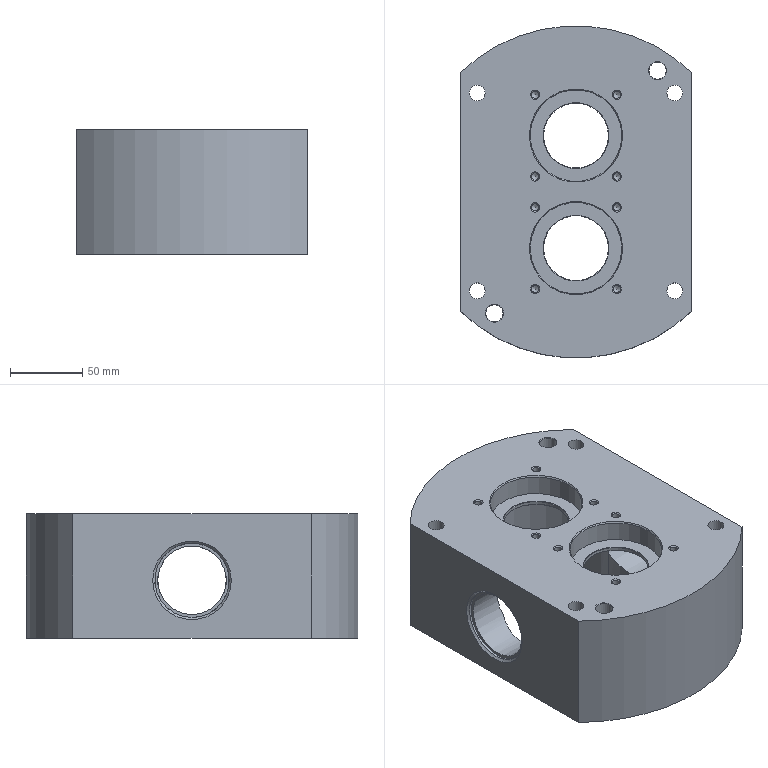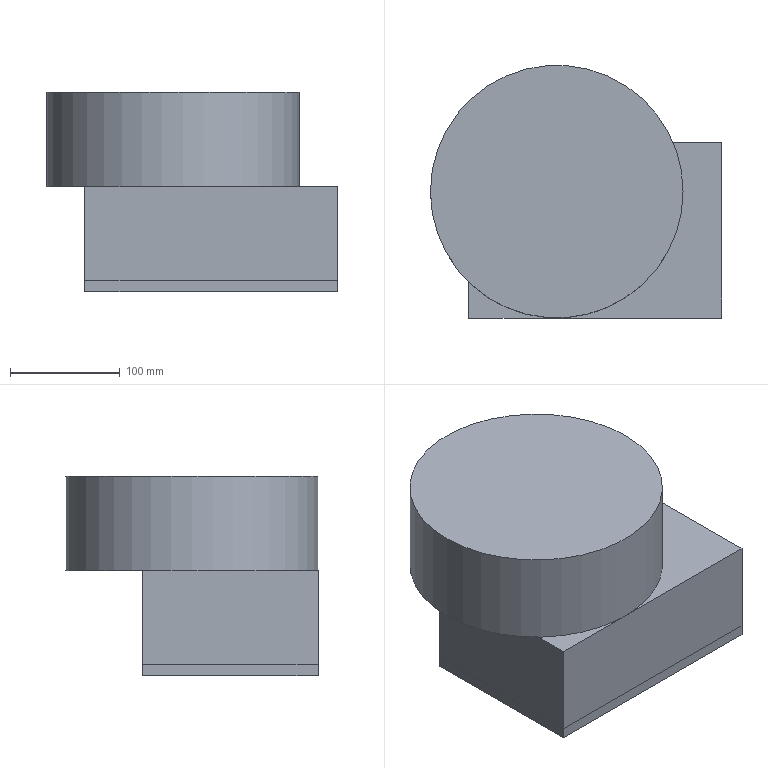CAM job | NX | 3+2 milling, drilling | part box 160 x 230 x 86 mm | stock box 265 x 230 x 182 mm
Tools:
number,name,description,diameter,corner_radius,flute_length,length,flutes
2,D50,Milling Tool-5 Parameters,50.0,0.0,50.0,75.0,2
10,D10,Milling Tool-5 Parameters,10.0,0.0,50.0,75.0,2
11,D10JING,Milling Tool-5 Parameters,10.0,0.0,50.0,75.0,2
7,D6A45,Milling Tool-5 Parameters,6.0,0.0,50.0,75.0,2
1,ZXZ,Milling Tool-5 Parameters,6.0,0.0,50.0,75.0,2
9,11.0ZT,Drilling Tool,11.0,0.0,35.0,50.0,2
8,11.8ZT,Drilling Tool,11.8,0.0,35.0,50.0,2
18,12.0JD,Milling Tool-5 Parameters,8.0,0.0,30.0,30.0,4
15,5.0ZT,Drilling Tool,5.0,0.0,35.0,50.0,2
16,6.8ZT,Drilling Tool,6.8,0.0,35.0,50.0,2
5,D25R0.5,Milling Tool-5 Parameters,25.0,0.5,50.0,75.0,2
12,D12,Milling Tool-5 Parameters,12.0,0.0,50.0,75.0,2
14,M6,Milling Tool-5 Parameters,5.0,0.0,30.0,30.0,4
18,M8,Milling Tool-5 Parameters,6.8,0.0,30.0,30.0,4
Operations:
program,operation,operation_type,tool,method,geometry_group,spindle_rpm,surface_speed,feed_per_tooth,feed_cut,feed_plunge,cut_length_mm,path_length_mm,cut_time_min,machine_time_min
1,FLOOR_WALL,VolumeBased25DMillingOperation,D50,METHOD,A,1200.0,188.0,0.8333,2000.0,1000.0,83660.764,101099.88,42.13,43.874
1,FLOOR_WALL_COPY,VolumeBased25DMillingOperation,D50,METHOD,A,2500.0,392.0,0.2,1000.0,1000.0,1038.906,1162.906,1.039,1.051
1,HOLE_MILLING,CylinderMilling,D10,METHOD,A,3000.0,94.0,0.3667,2200.0,100.0,6416.122,6548.622,2.916,2.93
1,HOLE_MILLING_COPY,CylinderMilling,D10,METHOD,A,3000.0,94.0,0.3667,2200.0,100.0,7693.753,7859.253,3.497,3.514
1,HOLE_MILLING_COPY_1,CylinderMilling,D10JING,METHOD,A,5000.0,157.0,0.1,1000.0,100.0,175.612,311.612,0.1756,0.1892
1,HOLE_MILLING_COPY_1_COPY,CylinderMilling,D10JING,METHOD,A,5000.0,157.0,0.1,1000.0,100.0,163.983,359.983,0.164,0.1836
1,PLANAR_MILL,PlanarMilling,D6A45,METHOD,A,7500.0,141.0,0.0833,1250.0,100.0,350.346,691.746,0.2803,0.3144
1,PLANAR_MILL_COPY,PlanarMilling,D6A45,METHOD,A,7500.0,141.0,0.0833,1250.0,100.0,483.313,611.313,0.3867,0.3995
2,DRILLING,Operation,ZXZ,METHOD,B,5000.0,94.0,0.025,250.0,0.0,64.0,820.526,0.256,0.3317
2,DRILLING_COPY,Operation,11.0ZT,METHOD,B,2000.0,56.0,0.0375,150.0,0.0,377.219,1234.536,2.515,2.6
2,DRILLING_COPY_COPY,Operation,11.8ZT,METHOD,B,2000.0,56.0,0.0375,150.0,0.0,188.09,641.67,1.254,1.299
2,DRILLING_COPY_COPY_COPY,Operation,12.0JD,METHOD,B,800.0,20.0,0.0125,40.0,0.0,179.0,623.49,4.475,4.519
2,DRILLING_COPY_COPY_1,Operation,5.0ZT,METHOD,B,2000.0,56.0,0.0375,150.0,0.0,140.017,687.555,0.9334,0.9882
2,DRILLING_COPY_2_COPY_COPY_1_COPY,Operation,M6,METHOD,B,200.0,3.0,0.0013,1.0,0.0,128.0,663.521,128.0,128.054
2,HOLE_MILLING_COPY_COPY,CylinderMilling,D10,METHOD,B,3000.0,94.0,0.3667,2200.0,100.0,24671.677,24898.677,11.214,11.237
2,HOLE_MILLING_COPY_COPY_COPY,CylinderMilling,D10,METHOD,B,3000.0,94.0,0.3667,2200.0,100.0,10167.626,10429.626,4.622,4.648
2,ZLEVEL_PROFILE,ZLevelMilling,D10JING,METHOD,B,5000.0,157.0,0.125,1250.0,100.0,239.51,498.755,0.1916,0.2175
2,PLANAR_MILL_COPY_COPY,PlanarMilling,D6A45,METHOD,B,7500.0,141.0,0.0833,1250.0,100.0,807.404,2282.468,0.6459,0.7934
2,PLANAR_MILL_COPY_COPY_COPY,PlanarMilling,D6A45,METHOD,B,7500.0,141.0,0.0833,1250.0,100.0,287.856,536.813,0.2303,0.2552
2,刀补,CylinderMilling,D10JING,METHOD,B,5000.0,157.0,0.1,1000.0,100.0,357.211,608.344,0.3572,0.3823
3,FLOOR_WALL_COPY_1,VolumeBased25DMillingOperation,D50,METHOD,C,1200.0,188.0,0.8333,2000.0,1000.0,48487.913,59439.44,24.331,25.426
3,FLOOR_WALL_COPY_COPY,VolumeBased25DMillingOperation,D50,METHOD,C,2500.0,392.0,0.2,1000.0,1000.0,1671.997,1725.997,1.672,1.677
3,DRILLING_COPY_1,Operation,ZXZ,METHOD,C,5000.0,94.0,0.025,250.0,0.0,24.0,577.424,0.096,0.1513
3,DRILLING_COPY_1_COPY,Operation,6.8ZT,METHOD,C,2000.0,42.0,0.05,200.0,0.0,210.258,949.939,1.051,1.125
3,DRILLING_COPY_2_COPY_COPY,Operation,M8,METHOD,C,200.0,4.0,0.0016,1.25,0.0,198.0,925.424,158.4,158.473
3,FLOOR_WALL_1,VolumeBased25DMillingOperation,D25R0.5,METHOD,C,2000.0,157.0,0.55,2200.0,1000.0,207221.659,221271.888,101.706,103.111
3,FLOOR_WALL_1_COPY_COPY,VolumeBased25DMillingOperation,D12,METHOD,C,4000.0,150.0,0.125,1000.0,500.0,3223.1,3413.5,3.229,3.248
3,HOLE_MILLING_1,CylinderMilling,D10,METHOD,C,3000.0,94.0,0.2667,1600.0,100.0,13986.943,14759.943,8.742,8.819
3,PLANAR_MILL_COPY_COPY_COPY_1,PlanarMilling,D6A45,METHOD,C,7500.0,141.0,0.0833,1250.0,100.0,951.218,2344.99,0.761,0.9004
3,刀补12,ZLevelMilling,D12,METHOD,C,5000.0,157.0,0.125,1250.0,100.0,1916.011,2493.417,1.533,1.591